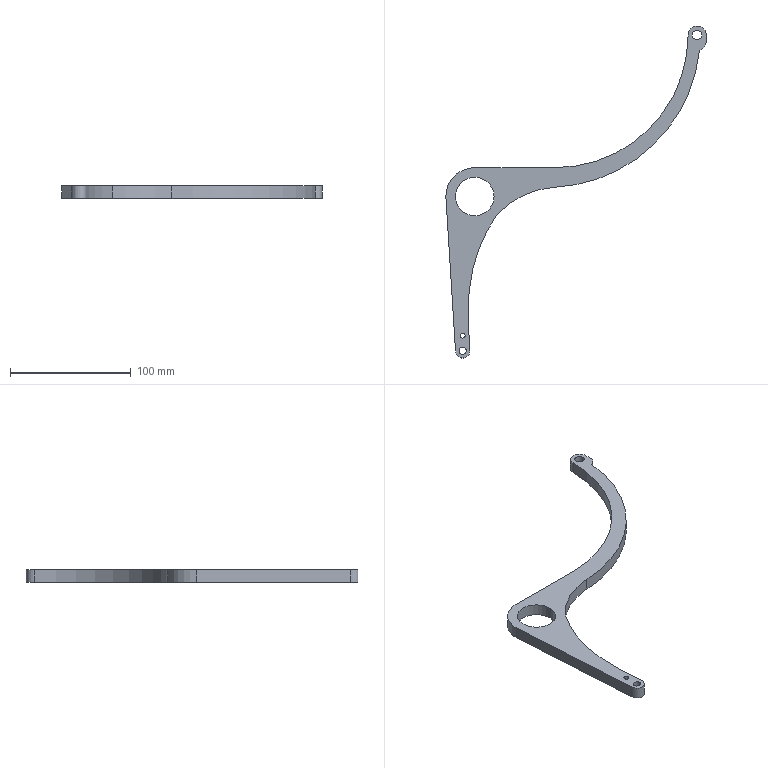Part | SolidWorks | features Extrusion 1 | 1 solid | 21 faces | box 216 x 275.5 x 10 mm | volume 64163 mm3 | cylinder 15 | plane 5 | spline 1 | commonest cylinder face diameters 4 x2 6 x2 7.838 x2 32 x2 12 x1 15 x1
STEP:
#1=CARTESIAN_POINT('',(-2.,12.5,10.));
#2=VERTEX_POINT('',#1);
#3=CARTESIAN_POINT('',(2.,12.5,10.));
#4=VERTEX_POINT('',#3);
#5=CARTESIAN_POINT('',(0.,12.5,10.));
#6=DIRECTION('',(0.,0.,1.));
#7=DIRECTION('',(1.,0.,0.));
#8=AXIS2_PLACEMENT_3D('',#5,#6,#7);
#9=CIRCLE('',#8,2.);
#10=EDGE_CURVE('',#2,#4,#9,.T.);
#11=ORIENTED_EDGE('',*,*,#10,.T.);
#12=CARTESIAN_POINT('',(2.,12.5,0.));
#13=VERTEX_POINT('',#12);
#14=CARTESIAN_POINT('',(2.,12.5,10.));
#15=DIRECTION('',(0.,0.,-1.));
#16=VECTOR('',#15,1000.);
#17=LINE('',#14,#16);
#18=EDGE_CURVE('',#4,#13,#17,.T.);
#19=ORIENTED_EDGE('',*,*,#18,.T.);
#20=CARTESIAN_POINT('',(-2.,12.5,0.));
#21=VERTEX_POINT('',#20);
#22=CARTESIAN_POINT('',(0.,12.5,0.));
#23=DIRECTION('',(0.,0.,1.));
#24=DIRECTION('',(1.,0.,0.));
#25=AXIS2_PLACEMENT_3D('',#22,#23,#24);
#26=CIRCLE('',#25,2.);
#27=EDGE_CURVE('',#21,#13,#26,.T.);
#28=ORIENTED_EDGE('',*,*,#27,.F.);
#29=CARTESIAN_POINT('',(-2.,12.5,10.));
#30=DIRECTION('',(0.,0.,-1.));
#31=VECTOR('',#30,1000.);
#32=LINE('',#29,#31);
#33=EDGE_CURVE('',#2,#21,#32,.T.);
#34=ORIENTED_EDGE('',*,*,#33,.F.);
#35=EDGE_LOOP('',(#11,#19,#28,#34));
#36=FACE_OUTER_BOUND('',#35,.T.);
#37=CARTESIAN_POINT('',(0.,12.5,10.));
#38=DIRECTION('',(0.,0.,-1.));
#39=DIRECTION('',(-1.,0.,0.));
#40=AXIS2_PLACEMENT_3D('',#37,#38,#39);
#41=CYLINDRICAL_SURFACE('',#40,2.);
#42=ADVANCED_FACE('',(#36),#41,.F.);
#43=CARTESIAN_POINT('',(190.581,262.,10.));
#44=VERTEX_POINT('',#43);
#45=CARTESIAN_POINT('',(198.419,262.,10.));
#46=VERTEX_POINT('',#45);
#47=CARTESIAN_POINT('',(194.5,262.,10.));
#48=DIRECTION('',(0.,0.,1.));
#49=DIRECTION('',(1.,0.,0.));
#50=AXIS2_PLACEMENT_3D('',#47,#48,#49);
#51=CIRCLE('',#50,3.919);
#52=EDGE_CURVE('',#44,#46,#51,.T.);
#53=ORIENTED_EDGE('',*,*,#52,.T.);
#54=CARTESIAN_POINT('',(198.419,262.,0.));
#55=VERTEX_POINT('',#54);
#56=CARTESIAN_POINT('',(198.419,262.,10.));
#57=DIRECTION('',(0.,0.,-1.));
#58=VECTOR('',#57,1000.);
#59=LINE('',#56,#58);
#60=EDGE_CURVE('',#46,#55,#59,.T.);
#61=ORIENTED_EDGE('',*,*,#60,.T.);
#62=CARTESIAN_POINT('',(190.581,262.,0.));
#63=VERTEX_POINT('',#62);
#64=CARTESIAN_POINT('',(194.5,262.,0.));
#65=DIRECTION('',(0.,0.,1.));
#66=DIRECTION('',(1.,0.,0.));
#67=AXIS2_PLACEMENT_3D('',#64,#65,#66);
#68=CIRCLE('',#67,3.919);
#69=EDGE_CURVE('',#63,#55,#68,.T.);
#70=ORIENTED_EDGE('',*,*,#69,.F.);
#71=CARTESIAN_POINT('',(190.581,262.,10.));
#72=DIRECTION('',(0.,0.,-1.));
#73=VECTOR('',#72,1000.);
#74=LINE('',#71,#73);
#75=EDGE_CURVE('',#44,#63,#74,.T.);
#76=ORIENTED_EDGE('',*,*,#75,.F.);
#77=EDGE_LOOP('',(#53,#61,#70,#76));
#78=FACE_OUTER_BOUND('',#77,.T.);
#79=CARTESIAN_POINT('',(194.5,262.,10.));
#80=DIRECTION('',(0.,0.,-1.));
#81=DIRECTION('',(-1.,0.,0.));
#82=AXIS2_PLACEMENT_3D('',#79,#80,#81);
#83=CYLINDRICAL_SURFACE('',#82,3.919);
#84=ADVANCED_FACE('',(#78),#83,.F.);
#85=CARTESIAN_POINT('',(-6.,128.,10.));
#86=VERTEX_POINT('',#85);
#87=CARTESIAN_POINT('',(26.,128.,10.));
#88=VERTEX_POINT('',#87);
#89=CARTESIAN_POINT('',(10.,128.,10.));
#90=DIRECTION('',(0.,0.,1.));
#91=DIRECTION('',(1.,0.,0.));
#92=AXIS2_PLACEMENT_3D('',#89,#90,#91);
#93=CIRCLE('',#92,16.);
#94=EDGE_CURVE('',#86,#88,#93,.T.);
#95=ORIENTED_EDGE('',*,*,#94,.T.);
#96=CARTESIAN_POINT('',(26.,128.,0.));
#97=VERTEX_POINT('',#96);
#98=CARTESIAN_POINT('',(26.,128.,10.));
#99=DIRECTION('',(0.,0.,-1.));
#100=VECTOR('',#99,1000.);
#101=LINE('',#98,#100);
#102=EDGE_CURVE('',#88,#97,#101,.T.);
#103=ORIENTED_EDGE('',*,*,#102,.T.);
#104=CARTESIAN_POINT('',(-6.,128.,0.));
#105=VERTEX_POINT('',#104);
#106=CARTESIAN_POINT('',(10.,128.,0.));
#107=DIRECTION('',(0.,0.,1.));
#108=DIRECTION('',(1.,0.,0.));
#109=AXIS2_PLACEMENT_3D('',#106,#107,#108);
#110=CIRCLE('',#109,16.);
#111=EDGE_CURVE('',#105,#97,#110,.T.);
#112=ORIENTED_EDGE('',*,*,#111,.F.);
#113=CARTESIAN_POINT('',(-6.,128.,10.));
#114=DIRECTION('',(0.,0.,-1.));
#115=VECTOR('',#114,1000.);
#116=LINE('',#113,#115);
#117=EDGE_CURVE('',#86,#105,#116,.T.);
#118=ORIENTED_EDGE('',*,*,#117,.F.);
#119=EDGE_LOOP('',(#95,#103,#112,#118));
#120=FACE_OUTER_BOUND('',#119,.T.);
#121=CARTESIAN_POINT('',(10.,128.,10.));
#122=DIRECTION('',(0.,0.,-1.));
#123=DIRECTION('',(-1.,0.,0.));
#124=AXIS2_PLACEMENT_3D('',#121,#122,#123);
#125=CYLINDRICAL_SURFACE('',#124,16.);
#126=ADVANCED_FACE('',(#120),#125,.F.);
#127=CARTESIAN_POINT('',(-3.,0.,10.));
#128=VERTEX_POINT('',#127);
#129=CARTESIAN_POINT('',(3.,0.,10.));
#130=VERTEX_POINT('',#129);
#131=CARTESIAN_POINT('',(0.,0.,10.));
#132=DIRECTION('',(0.,0.,1.));
#133=DIRECTION('',(1.,0.,0.));
#134=AXIS2_PLACEMENT_3D('',#131,#132,#133);
#135=CIRCLE('',#134,3.);
#136=EDGE_CURVE('',#128,#130,#135,.T.);
#137=ORIENTED_EDGE('',*,*,#136,.T.);
#138=CARTESIAN_POINT('',(3.,0.,0.));
#139=VERTEX_POINT('',#138);
#140=CARTESIAN_POINT('',(3.,0.,10.));
#141=DIRECTION('',(0.,0.,-1.));
#142=VECTOR('',#141,1000.);
#143=LINE('',#140,#142);
#144=EDGE_CURVE('',#130,#139,#143,.T.);
#145=ORIENTED_EDGE('',*,*,#144,.T.);
#146=CARTESIAN_POINT('',(-3.,0.,0.));
#147=VERTEX_POINT('',#146);
#148=CARTESIAN_POINT('',(0.,0.,0.));
#149=DIRECTION('',(0.,0.,1.));
#150=DIRECTION('',(1.,0.,0.));
#151=AXIS2_PLACEMENT_3D('',#148,#149,#150);
#152=CIRCLE('',#151,3.);
#153=EDGE_CURVE('',#147,#139,#152,.T.);
#154=ORIENTED_EDGE('',*,*,#153,.F.);
#155=CARTESIAN_POINT('',(-3.,0.,10.));
#156=DIRECTION('',(0.,0.,-1.));
#157=VECTOR('',#156,1000.);
#158=LINE('',#155,#157);
#159=EDGE_CURVE('',#128,#147,#158,.T.);
#160=ORIENTED_EDGE('',*,*,#159,.F.);
#161=EDGE_LOOP('',(#137,#145,#154,#160));
#162=FACE_OUTER_BOUND('',#161,.T.);
#163=CARTESIAN_POINT('',(0.,0.,10.));
#164=DIRECTION('',(0.,0.,-1.));
#165=DIRECTION('',(-1.,0.,0.));
#166=AXIS2_PLACEMENT_3D('',#163,#164,#165);
#167=CYLINDRICAL_SURFACE('',#166,3.);
#168=ADVANCED_FACE('',(#162),#167,.F.);
#169=ORIENTED_EDGE('',*,*,#52,.F.);
#170=CARTESIAN_POINT('',(194.5,262.,10.));
#171=DIRECTION('',(0.,0.,1.));
#172=DIRECTION('',(1.,0.,0.));
#173=AXIS2_PLACEMENT_3D('',#170,#171,#172);
#174=CIRCLE('',#173,3.919);
#175=EDGE_CURVE('',#46,#44,#174,.T.);
#176=ORIENTED_EDGE('',*,*,#175,.F.);
#177=EDGE_LOOP('',(#169,#176));
#178=FACE_BOUND('',#177,.T.);
#179=ORIENTED_EDGE('',*,*,#136,.F.);
#180=CARTESIAN_POINT('',(0.,0.,10.));
#181=DIRECTION('',(0.,0.,1.));
#182=DIRECTION('',(1.,0.,0.));
#183=AXIS2_PLACEMENT_3D('',#180,#181,#182);
#184=CIRCLE('',#183,3.);
#185=EDGE_CURVE('',#130,#128,#184,.T.);
#186=ORIENTED_EDGE('',*,*,#185,.F.);
#187=EDGE_LOOP('',(#179,#186));
#188=FACE_BOUND('',#187,.T.);
#189=CARTESIAN_POINT('',(10.,152.,10.));
#190=VERTEX_POINT('',#189);
#191=CARTESIAN_POINT('',(-14.,128.,10.));
#192=VERTEX_POINT('',#191);
#193=CARTESIAN_POINT('',(10.,128.,10.));
#194=DIRECTION('',(0.,0.,1.));
#195=DIRECTION('',(1.,0.,0.));
#196=AXIS2_PLACEMENT_3D('',#193,#194,#195);
#197=CIRCLE('',#196,24.);
#198=EDGE_CURVE('',#190,#192,#197,.T.);
#199=ORIENTED_EDGE('',*,*,#198,.T.);
#200=CARTESIAN_POINT('',(-6.,0.,10.));
#201=VERTEX_POINT('',#200);
#202=CARTESIAN_POINT('',(-14.,128.,10.));
#203=DIRECTION('',(0.06238,-0.9981,0.));
#204=VECTOR('',#203,1000.);
#205=LINE('',#202,#204);
#206=EDGE_CURVE('',#192,#201,#205,.T.);
#207=ORIENTED_EDGE('',*,*,#206,.T.);
#208=CARTESIAN_POINT('',(6.,0.,10.));
#209=VERTEX_POINT('',#208);
#210=CARTESIAN_POINT('',(0.,0.,10.));
#211=DIRECTION('',(0.,0.,1.));
#212=DIRECTION('',(1.,0.,0.));
#213=AXIS2_PLACEMENT_3D('',#210,#211,#212);
#214=CIRCLE('',#213,6.);
#215=EDGE_CURVE('',#201,#209,#214,.T.);
#216=ORIENTED_EDGE('',*,*,#215,.T.);
#217=CARTESIAN_POINT('',(28.005,112.131,10.));
#218=VERTEX_POINT('',#217);
#219=CARTESIAN_POINT('',(6.,0.,10.));
#220=CARTESIAN_POINT('',(1.589,45.681,10.));
#221=CARTESIAN_POINT('',(5.604,79.643,10.));
#222=CARTESIAN_POINT('',(28.005,112.131,10.));
#223=B_SPLINE_CURVE_WITH_KNOTS('',3,(#219,#220,#221,#222),.UNSPECIFIED.,.F.,.F.,(4,4),(0.,0.7882),.UNSPECIFIED.);
#224=EDGE_CURVE('',#209,#218,#223,.T.);
#225=ORIENTED_EDGE('',*,*,#224,.T.);
#226=CARTESIAN_POINT('',(77.,135.767,10.));
#227=VERTEX_POINT('',#226);
#228=CARTESIAN_POINT('',(80.543,65.825,10.));
#229=DIRECTION('',(0.,0.,-1.));
#230=DIRECTION('',(1.,0.,0.));
#231=AXIS2_PLACEMENT_3D('',#228,#229,#230);
#232=CIRCLE('',#231,70.032);
#233=EDGE_CURVE('',#218,#227,#232,.T.);
#234=ORIENTED_EDGE('',*,*,#233,.T.);
#235=CARTESIAN_POINT('',(196.38,249.495,10.));
#236=VERTEX_POINT('',#235);
#237=CARTESIAN_POINT('',(70.606,262.,10.));
#238=DIRECTION('',(0.,0.,1.));
#239=DIRECTION('',(1.,0.,0.));
#240=AXIS2_PLACEMENT_3D('',#237,#238,#239);
#241=CIRCLE('',#240,126.394);
#242=EDGE_CURVE('',#227,#236,#241,.T.);
#243=ORIENTED_EDGE('',*,*,#242,.T.);
#244=CARTESIAN_POINT('',(202.,257.,10.));
#245=VERTEX_POINT('',#244);
#246=CARTESIAN_POINT('',(194.179,257.,10.));
#247=DIRECTION('',(0.,0.,1.));
#248=DIRECTION('',(1.,0.,0.));
#249=AXIS2_PLACEMENT_3D('',#246,#247,#248);
#250=CIRCLE('',#249,7.821);
#251=EDGE_CURVE('',#236,#245,#250,.T.);
#252=ORIENTED_EDGE('',*,*,#251,.T.);
#253=CARTESIAN_POINT('',(202.,262.,10.));
#254=VERTEX_POINT('',#253);
#255=CARTESIAN_POINT('',(202.,262.,10.));
#256=DIRECTION('',(0.,1.,0.));
#257=VECTOR('',#256,1000.);
#258=LINE('',#255,#257);
#259=EDGE_CURVE('',#245,#254,#258,.T.);
#260=ORIENTED_EDGE('',*,*,#259,.T.);
#261=CARTESIAN_POINT('',(187.,262.,10.));
#262=VERTEX_POINT('',#261);
#263=CARTESIAN_POINT('',(194.5,262.,10.));
#264=DIRECTION('',(0.,0.,1.));
#265=DIRECTION('',(1.,0.,0.));
#266=AXIS2_PLACEMENT_3D('',#263,#264,#265);
#267=CIRCLE('',#266,7.5);
#268=EDGE_CURVE('',#254,#262,#267,.T.);
#269=ORIENTED_EDGE('',*,*,#268,.T.);
#270=CARTESIAN_POINT('',(77.,152.,10.));
#271=VERTEX_POINT('',#270);
#272=CARTESIAN_POINT('',(77.,262.,10.));
#273=DIRECTION('',(0.,0.,-1.));
#274=DIRECTION('',(1.,0.,0.));
#275=AXIS2_PLACEMENT_3D('',#272,#273,#274);
#276=CIRCLE('',#275,110.);
#277=EDGE_CURVE('',#262,#271,#276,.T.);
#278=ORIENTED_EDGE('',*,*,#277,.T.);
#279=CARTESIAN_POINT('',(10.,152.,10.));
#280=DIRECTION('',(-1.,0.,0.));
#281=VECTOR('',#280,1000.);
#282=LINE('',#279,#281);
#283=EDGE_CURVE('',#271,#190,#282,.T.);
#284=ORIENTED_EDGE('',*,*,#283,.T.);
#285=EDGE_LOOP('',(#199,#207,#216,#225,#234,#243,#252,#260,#269,#278,#284));
#286=FACE_OUTER_BOUND('',#285,.T.);
#287=ORIENTED_EDGE('',*,*,#94,.F.);
#288=CARTESIAN_POINT('',(10.,128.,10.));
#289=DIRECTION('',(0.,0.,1.));
#290=DIRECTION('',(1.,0.,0.));
#291=AXIS2_PLACEMENT_3D('',#288,#289,#290);
#292=CIRCLE('',#291,16.);
#293=EDGE_CURVE('',#88,#86,#292,.T.);
#294=ORIENTED_EDGE('',*,*,#293,.F.);
#295=EDGE_LOOP('',(#287,#294));
#296=FACE_BOUND('',#295,.T.);
#297=ORIENTED_EDGE('',*,*,#10,.F.);
#298=CARTESIAN_POINT('',(0.,12.5,10.));
#299=DIRECTION('',(0.,0.,1.));
#300=DIRECTION('',(1.,0.,0.));
#301=AXIS2_PLACEMENT_3D('',#298,#299,#300);
#302=CIRCLE('',#301,2.);
#303=EDGE_CURVE('',#4,#2,#302,.T.);
#304=ORIENTED_EDGE('',*,*,#303,.F.);
#305=EDGE_LOOP('',(#297,#304));
#306=FACE_BOUND('',#305,.T.);
#307=CARTESIAN_POINT('',(10.,128.,10.));
#308=DIRECTION('',(0.,0.,1.));
#309=DIRECTION('',(1.,0.,0.));
#310=AXIS2_PLACEMENT_3D('',#307,#308,#309);
#311=PLANE('',#310);
#312=ADVANCED_FACE('',(#178,#188,#286,#296,#306),#311,.T.);
#313=CARTESIAN_POINT('',(10.,152.,0.));
#314=VERTEX_POINT('',#313);
#315=CARTESIAN_POINT('',(-14.,128.,0.));
#316=VERTEX_POINT('',#315);
#317=CARTESIAN_POINT('',(10.,128.,0.));
#318=DIRECTION('',(0.,0.,1.));
#319=DIRECTION('',(1.,0.,0.));
#320=AXIS2_PLACEMENT_3D('',#317,#318,#319);
#321=CIRCLE('',#320,24.);
#322=EDGE_CURVE('',#314,#316,#321,.T.);
#323=ORIENTED_EDGE('',*,*,#322,.F.);
#324=CARTESIAN_POINT('',(77.,152.,0.));
#325=VERTEX_POINT('',#324);
#326=CARTESIAN_POINT('',(10.,152.,0.));
#327=DIRECTION('',(-1.,0.,0.));
#328=VECTOR('',#327,1000.);
#329=LINE('',#326,#328);
#330=EDGE_CURVE('',#325,#314,#329,.T.);
#331=ORIENTED_EDGE('',*,*,#330,.F.);
#332=CARTESIAN_POINT('',(187.,262.,0.));
#333=VERTEX_POINT('',#332);
#334=CARTESIAN_POINT('',(77.,262.,0.));
#335=DIRECTION('',(0.,0.,-1.));
#336=DIRECTION('',(1.,0.,0.));
#337=AXIS2_PLACEMENT_3D('',#334,#335,#336);
#338=CIRCLE('',#337,110.);
#339=EDGE_CURVE('',#333,#325,#338,.T.);
#340=ORIENTED_EDGE('',*,*,#339,.F.);
#341=CARTESIAN_POINT('',(202.,262.,0.));
#342=VERTEX_POINT('',#341);
#343=CARTESIAN_POINT('',(194.5,262.,0.));
#344=DIRECTION('',(0.,0.,1.));
#345=DIRECTION('',(1.,0.,0.));
#346=AXIS2_PLACEMENT_3D('',#343,#344,#345);
#347=CIRCLE('',#346,7.5);
#348=EDGE_CURVE('',#342,#333,#347,.T.);
#349=ORIENTED_EDGE('',*,*,#348,.F.);
#350=CARTESIAN_POINT('',(202.,257.,0.));
#351=VERTEX_POINT('',#350);
#352=CARTESIAN_POINT('',(202.,262.,0.));
#353=DIRECTION('',(0.,1.,0.));
#354=VECTOR('',#353,1000.);
#355=LINE('',#352,#354);
#356=EDGE_CURVE('',#351,#342,#355,.T.);
#357=ORIENTED_EDGE('',*,*,#356,.F.);
#358=CARTESIAN_POINT('',(196.38,249.495,0.));
#359=VERTEX_POINT('',#358);
#360=CARTESIAN_POINT('',(194.179,257.,0.));
#361=DIRECTION('',(0.,0.,1.));
#362=DIRECTION('',(1.,0.,0.));
#363=AXIS2_PLACEMENT_3D('',#360,#361,#362);
#364=CIRCLE('',#363,7.821);
#365=EDGE_CURVE('',#359,#351,#364,.T.);
#366=ORIENTED_EDGE('',*,*,#365,.F.);
#367=CARTESIAN_POINT('',(77.,135.767,0.));
#368=VERTEX_POINT('',#367);
#369=CARTESIAN_POINT('',(70.606,262.,0.));
#370=DIRECTION('',(0.,0.,1.));
#371=DIRECTION('',(1.,0.,0.));
#372=AXIS2_PLACEMENT_3D('',#369,#370,#371);
#373=CIRCLE('',#372,126.394);
#374=EDGE_CURVE('',#368,#359,#373,.T.);
#375=ORIENTED_EDGE('',*,*,#374,.F.);
#376=CARTESIAN_POINT('',(28.005,112.131,0.));
#377=VERTEX_POINT('',#376);
#378=CARTESIAN_POINT('',(80.543,65.825,0.));
#379=DIRECTION('',(0.,0.,-1.));
#380=DIRECTION('',(1.,0.,0.));
#381=AXIS2_PLACEMENT_3D('',#378,#379,#380);
#382=CIRCLE('',#381,70.032);
#383=EDGE_CURVE('',#377,#368,#382,.T.);
#384=ORIENTED_EDGE('',*,*,#383,.F.);
#385=CARTESIAN_POINT('',(6.,0.,0.));
#386=VERTEX_POINT('',#385);
#387=CARTESIAN_POINT('',(6.,0.,0.));
#388=CARTESIAN_POINT('',(1.589,45.681,0.));
#389=CARTESIAN_POINT('',(5.604,79.643,0.));
#390=CARTESIAN_POINT('',(28.005,112.131,0.));
#391=B_SPLINE_CURVE_WITH_KNOTS('',3,(#387,#388,#389,#390),.UNSPECIFIED.,.F.,.F.,(4,4),(0.,0.7882),.UNSPECIFIED.);
#392=EDGE_CURVE('',#386,#377,#391,.T.);
#393=ORIENTED_EDGE('',*,*,#392,.F.);
#394=CARTESIAN_POINT('',(-6.,0.,0.));
#395=VERTEX_POINT('',#394);
#396=CARTESIAN_POINT('',(0.,0.,0.));
#397=DIRECTION('',(0.,0.,1.));
#398=DIRECTION('',(1.,0.,0.));
#399=AXIS2_PLACEMENT_3D('',#396,#397,#398);
#400=CIRCLE('',#399,6.);
#401=EDGE_CURVE('',#395,#386,#400,.T.);
#402=ORIENTED_EDGE('',*,*,#401,.F.);
#403=CARTESIAN_POINT('',(-14.,128.,0.));
#404=DIRECTION('',(0.06238,-0.9981,0.));
#405=VECTOR('',#404,1000.);
#406=LINE('',#403,#405);
#407=EDGE_CURVE('',#316,#395,#406,.T.);
#408=ORIENTED_EDGE('',*,*,#407,.F.);
#409=EDGE_LOOP('',(#323,#331,#340,#349,#357,#366,#375,#384,#393,#402,#408));
#410=FACE_OUTER_BOUND('',#409,.T.);
#411=ORIENTED_EDGE('',*,*,#153,.T.);
#412=CARTESIAN_POINT('',(0.,0.,0.));
#413=DIRECTION('',(0.,0.,1.));
#414=DIRECTION('',(1.,0.,0.));
#415=AXIS2_PLACEMENT_3D('',#412,#413,#414);
#416=CIRCLE('',#415,3.);
#417=EDGE_CURVE('',#139,#147,#416,.T.);
#418=ORIENTED_EDGE('',*,*,#417,.T.);
#419=EDGE_LOOP('',(#411,#418));
#420=FACE_BOUND('',#419,.T.);
#421=ORIENTED_EDGE('',*,*,#111,.T.);
#422=CARTESIAN_POINT('',(10.,128.,0.));
#423=DIRECTION('',(0.,0.,1.));
#424=DIRECTION('',(1.,0.,0.));
#425=AXIS2_PLACEMENT_3D('',#422,#423,#424);
#426=CIRCLE('',#425,16.);
#427=EDGE_CURVE('',#97,#105,#426,.T.);
#428=ORIENTED_EDGE('',*,*,#427,.T.);
#429=EDGE_LOOP('',(#421,#428));
#430=FACE_BOUND('',#429,.T.);
#431=ORIENTED_EDGE('',*,*,#69,.T.);
#432=CARTESIAN_POINT('',(194.5,262.,0.));
#433=DIRECTION('',(0.,0.,1.));
#434=DIRECTION('',(1.,0.,0.));
#435=AXIS2_PLACEMENT_3D('',#432,#433,#434);
#436=CIRCLE('',#435,3.919);
#437=EDGE_CURVE('',#55,#63,#436,.T.);
#438=ORIENTED_EDGE('',*,*,#437,.T.);
#439=EDGE_LOOP('',(#431,#438));
#440=FACE_BOUND('',#439,.T.);
#441=ORIENTED_EDGE('',*,*,#27,.T.);
#442=CARTESIAN_POINT('',(0.,12.5,0.));
#443=DIRECTION('',(0.,0.,1.));
#444=DIRECTION('',(1.,0.,0.));
#445=AXIS2_PLACEMENT_3D('',#442,#443,#444);
#446=CIRCLE('',#445,2.);
#447=EDGE_CURVE('',#13,#21,#446,.T.);
#448=ORIENTED_EDGE('',*,*,#447,.T.);
#449=EDGE_LOOP('',(#441,#448));
#450=FACE_BOUND('',#449,.T.);
#451=CARTESIAN_POINT('',(10.,128.,0.));
#452=DIRECTION('',(0.,0.,1.));
#453=DIRECTION('',(1.,0.,0.));
#454=AXIS2_PLACEMENT_3D('',#451,#452,#453);
#455=PLANE('',#454);
#456=ADVANCED_FACE('',(#410,#420,#430,#440,#450),#455,.F.);
#457=ORIENTED_EDGE('',*,*,#322,.T.);
#458=CARTESIAN_POINT('',(-14.,128.,10.));
#459=DIRECTION('',(0.,0.,-1.));
#460=VECTOR('',#459,1000.);
#461=LINE('',#458,#460);
#462=EDGE_CURVE('',#192,#316,#461,.T.);
#463=ORIENTED_EDGE('',*,*,#462,.F.);
#464=ORIENTED_EDGE('',*,*,#198,.F.);
#465=CARTESIAN_POINT('',(10.,152.,10.));
#466=DIRECTION('',(0.,0.,-1.));
#467=VECTOR('',#466,1000.);
#468=LINE('',#465,#467);
#469=EDGE_CURVE('',#190,#314,#468,.T.);
#470=ORIENTED_EDGE('',*,*,#469,.T.);
#471=EDGE_LOOP('',(#457,#463,#464,#470));
#472=FACE_OUTER_BOUND('',#471,.T.);
#473=CARTESIAN_POINT('',(10.,128.,10.));
#474=DIRECTION('',(0.,0.,-1.));
#475=DIRECTION('',(-1.,0.,0.));
#476=AXIS2_PLACEMENT_3D('',#473,#474,#475);
#477=CYLINDRICAL_SURFACE('',#476,24.);
#478=ADVANCED_FACE('',(#472),#477,.T.);
#479=ORIENTED_EDGE('',*,*,#407,.T.);
#480=CARTESIAN_POINT('',(-6.,0.,10.));
#481=DIRECTION('',(0.,0.,-1.));
#482=VECTOR('',#481,1000.);
#483=LINE('',#480,#482);
#484=EDGE_CURVE('',#201,#395,#483,.T.);
#485=ORIENTED_EDGE('',*,*,#484,.F.);
#486=ORIENTED_EDGE('',*,*,#206,.F.);
#487=ORIENTED_EDGE('',*,*,#462,.T.);
#488=EDGE_LOOP('',(#479,#485,#486,#487));
#489=FACE_OUTER_BOUND('',#488,.T.);
#490=CARTESIAN_POINT('',(-14.,128.,10.));
#491=DIRECTION('',(0.9981,0.06238,0.));
#492=DIRECTION('',(-0.06238,0.9981,0.));
#493=AXIS2_PLACEMENT_3D('',#490,#491,#492);
#494=PLANE('',#493);
#495=ADVANCED_FACE('',(#489),#494,.F.);
#496=ORIENTED_EDGE('',*,*,#401,.T.);
#497=CARTESIAN_POINT('',(6.,0.,10.));
#498=DIRECTION('',(0.,0.,-1.));
#499=VECTOR('',#498,1000.);
#500=LINE('',#497,#499);
#501=EDGE_CURVE('',#209,#386,#500,.T.);
#502=ORIENTED_EDGE('',*,*,#501,.F.);
#503=ORIENTED_EDGE('',*,*,#215,.F.);
#504=ORIENTED_EDGE('',*,*,#484,.T.);
#505=EDGE_LOOP('',(#496,#502,#503,#504));
#506=FACE_OUTER_BOUND('',#505,.T.);
#507=CARTESIAN_POINT('',(0.,0.,10.));
#508=DIRECTION('',(0.,0.,-1.));
#509=DIRECTION('',(-1.,0.,0.));
#510=AXIS2_PLACEMENT_3D('',#507,#508,#509);
#511=CYLINDRICAL_SURFACE('',#510,6.);
#512=ADVANCED_FACE('',(#506),#511,.T.);
#513=ORIENTED_EDGE('',*,*,#392,.T.);
#514=CARTESIAN_POINT('',(28.005,112.131,10.));
#515=DIRECTION('',(0.,0.,-1.));
#516=VECTOR('',#515,1000.);
#517=LINE('',#514,#516);
#518=EDGE_CURVE('',#218,#377,#517,.T.);
#519=ORIENTED_EDGE('',*,*,#518,.F.);
#520=ORIENTED_EDGE('',*,*,#224,.F.);
#521=ORIENTED_EDGE('',*,*,#501,.T.);
#522=EDGE_LOOP('',(#513,#519,#520,#521));
#523=FACE_OUTER_BOUND('',#522,.T.);
#524=CARTESIAN_POINT('',(6.,0.,10.));
#525=CARTESIAN_POINT('',(6.,0.,0.));
#526=CARTESIAN_POINT('',(1.589,45.681,10.));
#527=CARTESIAN_POINT('',(1.589,45.681,0.));
#528=CARTESIAN_POINT('',(5.604,79.643,10.));
#529=CARTESIAN_POINT('',(5.604,79.643,0.));
#530=CARTESIAN_POINT('',(28.005,112.131,10.));
#531=CARTESIAN_POINT('',(28.005,112.131,0.));
#532=B_SPLINE_SURFACE_WITH_KNOTS('',3,1,((#524,#525),(#526,#527),(#528,#529),(#530,#531)),.UNSPECIFIED.,.F.,.F.,.F.,(4,4),(2,2),(0.,0.7882),(0.,1.),.UNSPECIFIED.);
#533=ADVANCED_FACE('',(#523),#532,.F.);
#534=ORIENTED_EDGE('',*,*,#383,.T.);
#535=CARTESIAN_POINT('',(77.,135.767,10.));
#536=DIRECTION('',(0.,0.,-1.));
#537=VECTOR('',#536,1000.);
#538=LINE('',#535,#537);
#539=EDGE_CURVE('',#227,#368,#538,.T.);
#540=ORIENTED_EDGE('',*,*,#539,.F.);
#541=ORIENTED_EDGE('',*,*,#233,.F.);
#542=ORIENTED_EDGE('',*,*,#518,.T.);
#543=EDGE_LOOP('',(#534,#540,#541,#542));
#544=FACE_OUTER_BOUND('',#543,.T.);
#545=CARTESIAN_POINT('',(80.543,65.825,10.));
#546=DIRECTION('',(0.,0.,-1.));
#547=DIRECTION('',(-1.,0.,0.));
#548=AXIS2_PLACEMENT_3D('',#545,#546,#547);
#549=CYLINDRICAL_SURFACE('',#548,70.032);
#550=ADVANCED_FACE('',(#544),#549,.F.);
#551=ORIENTED_EDGE('',*,*,#374,.T.);
#552=CARTESIAN_POINT('',(196.38,249.495,10.));
#553=DIRECTION('',(0.,0.,-1.));
#554=VECTOR('',#553,1000.);
#555=LINE('',#552,#554);
#556=EDGE_CURVE('',#236,#359,#555,.T.);
#557=ORIENTED_EDGE('',*,*,#556,.F.);
#558=ORIENTED_EDGE('',*,*,#242,.F.);
#559=ORIENTED_EDGE('',*,*,#539,.T.);
#560=EDGE_LOOP('',(#551,#557,#558,#559));
#561=FACE_OUTER_BOUND('',#560,.T.);
#562=CARTESIAN_POINT('',(70.606,262.,10.));
#563=DIRECTION('',(0.,0.,-1.));
#564=DIRECTION('',(-1.,0.,0.));
#565=AXIS2_PLACEMENT_3D('',#562,#563,#564);
#566=CYLINDRICAL_SURFACE('',#565,126.394);
#567=ADVANCED_FACE('',(#561),#566,.T.);
#568=ORIENTED_EDGE('',*,*,#365,.T.);
#569=CARTESIAN_POINT('',(202.,257.,10.));
#570=DIRECTION('',(0.,0.,-1.));
#571=VECTOR('',#570,1000.);
#572=LINE('',#569,#571);
#573=EDGE_CURVE('',#245,#351,#572,.T.);
#574=ORIENTED_EDGE('',*,*,#573,.F.);
#575=ORIENTED_EDGE('',*,*,#251,.F.);
#576=ORIENTED_EDGE('',*,*,#556,.T.);
#577=EDGE_LOOP('',(#568,#574,#575,#576));
#578=FACE_OUTER_BOUND('',#577,.T.);
#579=CARTESIAN_POINT('',(194.179,257.,10.));
#580=DIRECTION('',(0.,0.,-1.));
#581=DIRECTION('',(-1.,0.,0.));
#582=AXIS2_PLACEMENT_3D('',#579,#580,#581);
#583=CYLINDRICAL_SURFACE('',#582,7.821);
#584=ADVANCED_FACE('',(#578),#583,.T.);
#585=ORIENTED_EDGE('',*,*,#356,.T.);
#586=CARTESIAN_POINT('',(202.,262.,10.));
#587=DIRECTION('',(0.,0.,-1.));
#588=VECTOR('',#587,1000.);
#589=LINE('',#586,#588);
#590=EDGE_CURVE('',#254,#342,#589,.T.);
#591=ORIENTED_EDGE('',*,*,#590,.F.);
#592=ORIENTED_EDGE('',*,*,#259,.F.);
#593=ORIENTED_EDGE('',*,*,#573,.T.);
#594=EDGE_LOOP('',(#585,#591,#592,#593));
#595=FACE_OUTER_BOUND('',#594,.T.);
#596=CARTESIAN_POINT('',(202.,262.,10.));
#597=DIRECTION('',(-1.,0.,0.));
#598=DIRECTION('',(0.,0.,1.));
#599=AXIS2_PLACEMENT_3D('',#596,#597,#598);
#600=PLANE('',#599);
#601=ADVANCED_FACE('',(#595),#600,.F.);
#602=ORIENTED_EDGE('',*,*,#348,.T.);
#603=CARTESIAN_POINT('',(187.,262.,10.));
#604=DIRECTION('',(0.,0.,-1.));
#605=VECTOR('',#604,1000.);
#606=LINE('',#603,#605);
#607=EDGE_CURVE('',#262,#333,#606,.T.);
#608=ORIENTED_EDGE('',*,*,#607,.F.);
#609=ORIENTED_EDGE('',*,*,#268,.F.);
#610=ORIENTED_EDGE('',*,*,#590,.T.);
#611=EDGE_LOOP('',(#602,#608,#609,#610));
#612=FACE_OUTER_BOUND('',#611,.T.);
#613=CARTESIAN_POINT('',(194.5,262.,10.));
#614=DIRECTION('',(0.,0.,-1.));
#615=DIRECTION('',(-1.,0.,0.));
#616=AXIS2_PLACEMENT_3D('',#613,#614,#615);
#617=CYLINDRICAL_SURFACE('',#616,7.5);
#618=ADVANCED_FACE('',(#612),#617,.T.);
#619=ORIENTED_EDGE('',*,*,#339,.T.);
#620=CARTESIAN_POINT('',(77.,152.,10.));
#621=DIRECTION('',(0.,0.,-1.));
#622=VECTOR('',#621,1000.);
#623=LINE('',#620,#622);
#624=EDGE_CURVE('',#271,#325,#623,.T.);
#625=ORIENTED_EDGE('',*,*,#624,.F.);
#626=ORIENTED_EDGE('',*,*,#277,.F.);
#627=ORIENTED_EDGE('',*,*,#607,.T.);
#628=EDGE_LOOP('',(#619,#625,#626,#627));
#629=FACE_OUTER_BOUND('',#628,.T.);
#630=CARTESIAN_POINT('',(77.,262.,10.));
#631=DIRECTION('',(0.,0.,-1.));
#632=DIRECTION('',(-1.,0.,0.));
#633=AXIS2_PLACEMENT_3D('',#630,#631,#632);
#634=CYLINDRICAL_SURFACE('',#633,110.);
#635=ADVANCED_FACE('',(#629),#634,.F.);
#636=ORIENTED_EDGE('',*,*,#330,.T.);
#637=ORIENTED_EDGE('',*,*,#469,.F.);
#638=ORIENTED_EDGE('',*,*,#283,.F.);
#639=ORIENTED_EDGE('',*,*,#624,.T.);
#640=EDGE_LOOP('',(#636,#637,#638,#639));
#641=FACE_OUTER_BOUND('',#640,.T.);
#642=CARTESIAN_POINT('',(10.,152.,10.));
#643=DIRECTION('',(0.,-1.,0.));
#644=DIRECTION('',(1.,0.,0.));
#645=AXIS2_PLACEMENT_3D('',#642,#643,#644);
#646=PLANE('',#645);
#647=ADVANCED_FACE('',(#641),#646,.F.);
#648=ORIENTED_EDGE('',*,*,#144,.F.);
#649=ORIENTED_EDGE('',*,*,#185,.T.);
#650=ORIENTED_EDGE('',*,*,#159,.T.);
#651=ORIENTED_EDGE('',*,*,#417,.F.);
#652=EDGE_LOOP('',(#648,#649,#650,#651));
#653=FACE_OUTER_BOUND('',#652,.T.);
#654=CARTESIAN_POINT('',(0.,0.,10.));
#655=DIRECTION('',(0.,0.,-1.));
#656=DIRECTION('',(-1.,0.,0.));
#657=AXIS2_PLACEMENT_3D('',#654,#655,#656);
#658=CYLINDRICAL_SURFACE('',#657,3.);
#659=ADVANCED_FACE('',(#653),#658,.F.);
#660=ORIENTED_EDGE('',*,*,#102,.F.);
#661=ORIENTED_EDGE('',*,*,#293,.T.);
#662=ORIENTED_EDGE('',*,*,#117,.T.);
#663=ORIENTED_EDGE('',*,*,#427,.F.);
#664=EDGE_LOOP('',(#660,#661,#662,#663));
#665=FACE_OUTER_BOUND('',#664,.T.);
#666=CARTESIAN_POINT('',(10.,128.,10.));
#667=DIRECTION('',(0.,0.,-1.));
#668=DIRECTION('',(-1.,0.,0.));
#669=AXIS2_PLACEMENT_3D('',#666,#667,#668);
#670=CYLINDRICAL_SURFACE('',#669,16.);
#671=ADVANCED_FACE('',(#665),#670,.F.);
#672=ORIENTED_EDGE('',*,*,#60,.F.);
#673=ORIENTED_EDGE('',*,*,#175,.T.);
#674=ORIENTED_EDGE('',*,*,#75,.T.);
#675=ORIENTED_EDGE('',*,*,#437,.F.);
#676=EDGE_LOOP('',(#672,#673,#674,#675));
#677=FACE_OUTER_BOUND('',#676,.T.);
#678=CARTESIAN_POINT('',(194.5,262.,10.));
#679=DIRECTION('',(0.,0.,-1.));
#680=DIRECTION('',(-1.,0.,0.));
#681=AXIS2_PLACEMENT_3D('',#678,#679,#680);
#682=CYLINDRICAL_SURFACE('',#681,3.919);
#683=ADVANCED_FACE('',(#677),#682,.F.);
#684=ORIENTED_EDGE('',*,*,#18,.F.);
#685=ORIENTED_EDGE('',*,*,#303,.T.);
#686=ORIENTED_EDGE('',*,*,#33,.T.);
#687=ORIENTED_EDGE('',*,*,#447,.F.);
#688=EDGE_LOOP('',(#684,#685,#686,#687));
#689=FACE_OUTER_BOUND('',#688,.T.);
#690=CARTESIAN_POINT('',(0.,12.5,10.));
#691=DIRECTION('',(0.,0.,-1.));
#692=DIRECTION('',(-1.,0.,0.));
#693=AXIS2_PLACEMENT_3D('',#690,#691,#692);
#694=CYLINDRICAL_SURFACE('',#693,2.);
#695=ADVANCED_FACE('',(#689),#694,.F.);
#696=CLOSED_SHELL('',(#42,#84,#126,#168,#312,#456,#478,#495,#512,#533,#550,#567,#584,#601,#618,#635,#647,#659,#671,#683,#695));
#697=MANIFOLD_SOLID_BREP('',#696);
#698=CARTESIAN_POINT('',(0.,0.,0.));
#699=DIRECTION('',(0.,0.,1.));
#700=DIRECTION('',(1.,0.,0.));
#701=AXIS2_PLACEMENT_3D('',#698,#699,#700);
#702=(LENGTH_UNIT()NAMED_UNIT(*)SI_UNIT(.MILLI.,.METRE.));
#703=UNCERTAINTY_MEASURE_WITH_UNIT(LENGTH_MEASURE(0.00001),#702,'','');
#704=(NAMED_UNIT(*)PLANE_ANGLE_UNIT()SI_UNIT($,.RADIAN.));
#705=(NAMED_UNIT(*)SI_UNIT($,.STERADIAN.)SOLID_ANGLE_UNIT());
#706=(GEOMETRIC_REPRESENTATION_CONTEXT(3)GLOBAL_UNCERTAINTY_ASSIGNED_CONTEXT((#703))GLOBAL_UNIT_ASSIGNED_CONTEXT((#702,#704,#705))REPRESENTATION_CONTEXT('',''));
#707=ADVANCED_BREP_SHAPE_REPRESENTATION('',(#697,#701),#706);